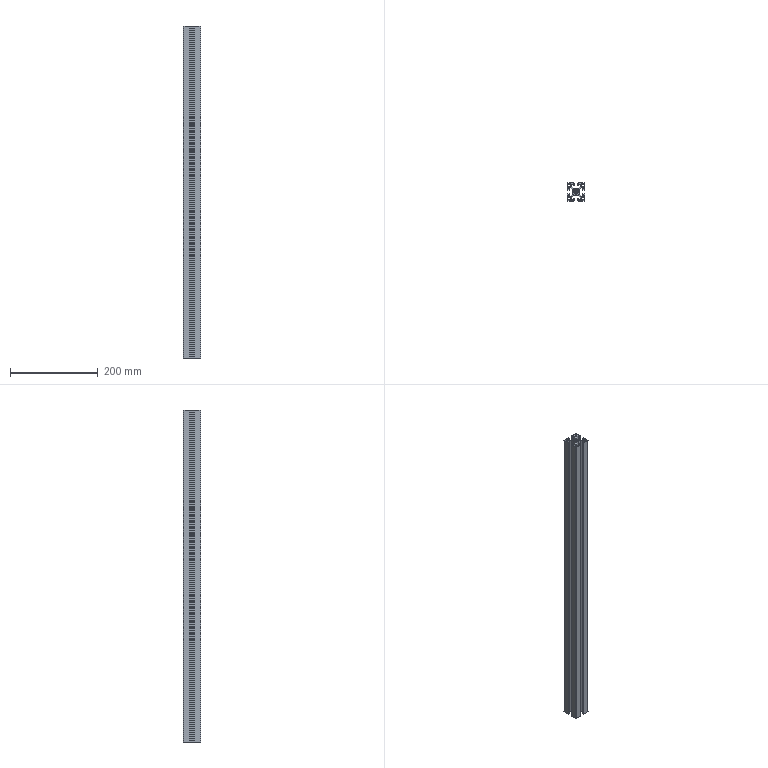Part | SolidWorks | features BaseBody 1, MoveFace 1 | 1 solid | 179 faces | box 40 x 40 x 757 mm | volume 405679 mm3 | plane 130 | cylinder 49 | commonest cylinder face diameters 0.6 x24 2 x8 10 x8 6.8 x5 3 x4